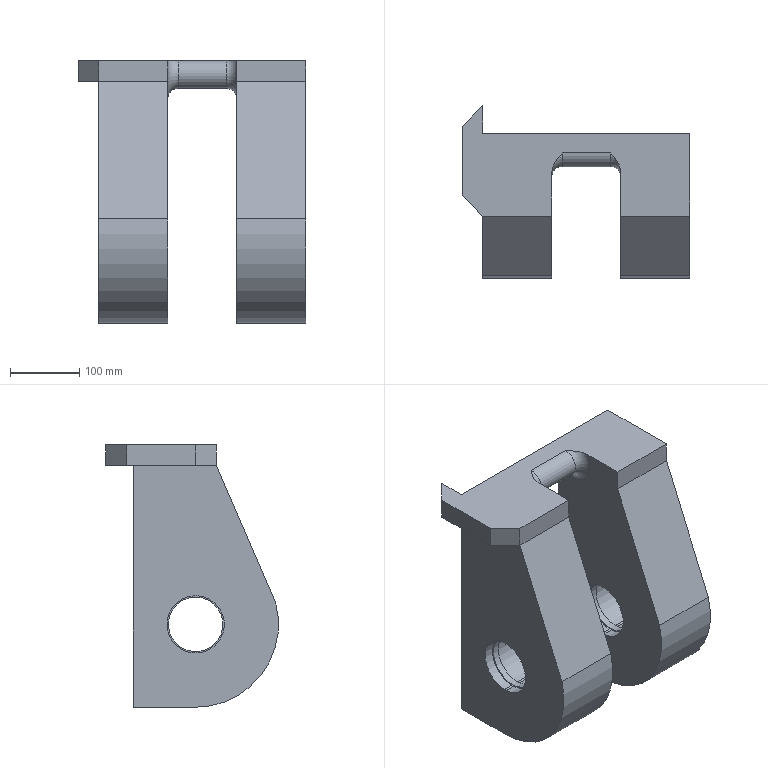Part | NX | features solid 2 | 1 solid | 81 faces | box 330 x 250 x 380 mm | volume 12163747 mm3 | plane 58 | cylinder 21 | torus 2 | commonest cylinder face diameters 83 x12 79 x4 30 x2 240 x2 40 x1